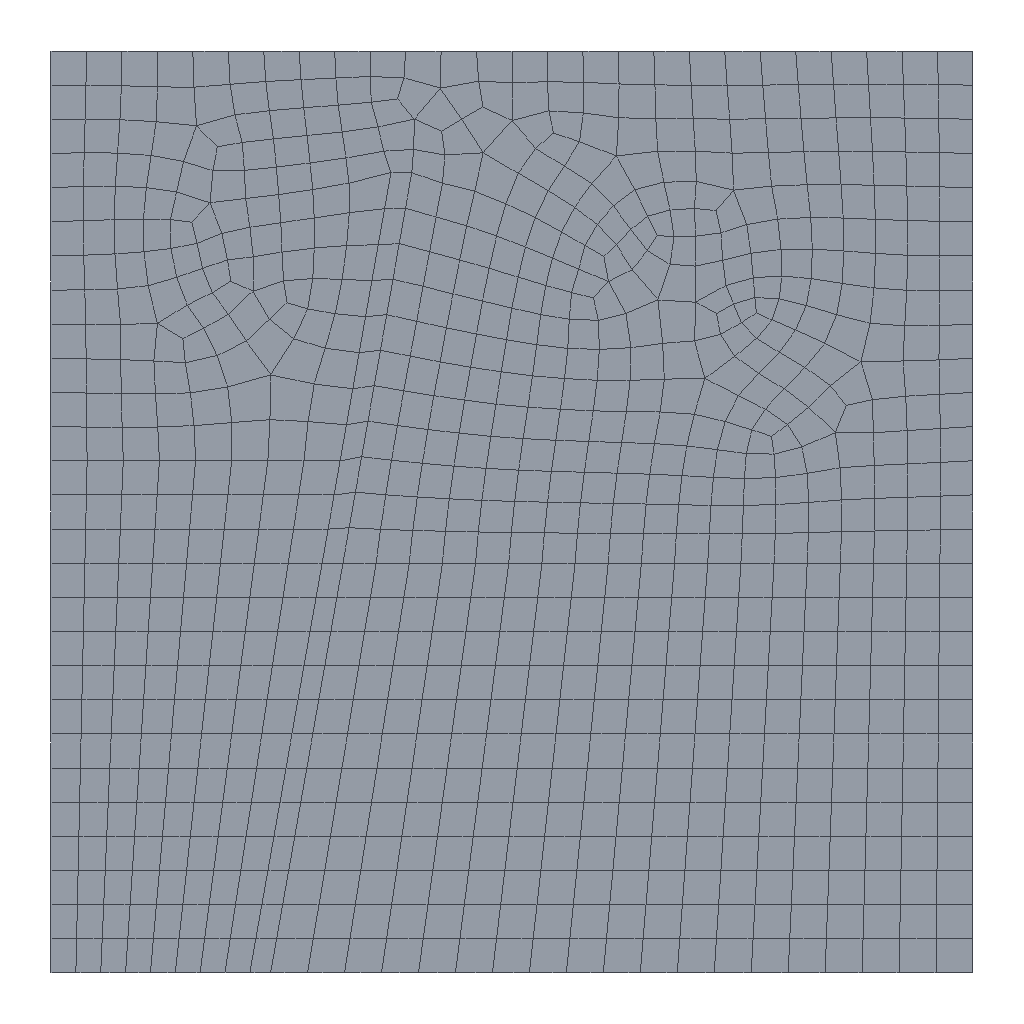Simulation study | abaqus
Set-up summary:
category,name,step,type,value,unit,region
solver,abaqus
solver,version,,,Abaqus/Standard 2020
units,not stated in the deck,,not stated
analysis,deck,,soils,soils
load_step,Step-1,Step-1,soils
load_step,requested,,,1
mesh,nodes,,,855
mesh,elements,,,800
element_type,CPE4P,,plane,800
load,load commands in deck,,count,3
bc,support commands in deck,,count,4
material,CHUSHUI,,in results
material,DUANCENG,,in results
material,SOIL,,in results
check,setup vs results,,match,"per instance, exact: element labels, types and connectivity; labels of the nodes the elements use; coordinates of those nodes at SINGLE_PRECISION in 1 of 1 instance(s)"
Abaqus input file, long lists of numbers shortened:
*Heading
** Job name: Job-2 Model name: Model-1-Copy
** Generated by: Abaqus/CAE 2020
*Preprint, echo=NO, model=NO, history=NO, contact=NO
**
** PARTS
**
*Part, name=Part-1
*Node
      1,   264.619,        -500.
      2,           0.,        -500.
** (853 more lines like these left out)
*Element, type=CPE4P
 1,   1,  17, 205,  52
 2,  17,  18, 206, 205
** (798 more lines like these left out)
*Nset, nset=Set-1
  1,  5, 53, 54
*Elset, elset=Set-1
 104, 112, 120, 133, 134, 135
*Nset, nset=Set-2
   1,   2,   3,   4,   5,   6,   7,   8,   9,  10,  11,  14,  15,  16,  17,  18
  19,  20,  21,  22,  23,  24,  25,  26,  27,  28,  29,  30,  31,  32,  33,  34
** (37 more lines like these left out)
*Elset, elset=Set-2
   1,   2,   3,   4,   5,   6,   7,   8,   9,  10,  11,  12,  13,  14,  15,  16
  17,  18,  19,  20,  21,  22,  23,  24,  25,  26,  27,  28,  29,  30,  31,  32
** (33 more lines like these left out)
*Nset, nset=Set-3
   1,   2,   5,   6,   8,   9,  12,  14,  17,  18,  19,  20,  21,  22,  23,  53
  54,  55,  56,  57,  58,  59,  60,  61,  62,  63,  72,  73,  91,  92,  93,  94
** (6 more lines like these left out)
*Elset, elset=Set-3
  97,  98,  99, 100, 101, 102, 103, 104, 105, 106, 107, 108, 109, 110, 111, 112
 113, 114, 115, 116, 117, 118, 119, 120, 315, 316, 317, 318, 319, 320, 321, 322
** (4 more lines like these left out)
*Nset, nset=Set-4
   7,   8,  12,  13,  64,  65,  66,  67,  68,  69,  70,  71,  91,  92,  93,  94
  95,  96,  97,  98,  99, 100, 101, 102, 103, 104, 105, 106, 107, 108, 109, 110
** (11 more lines like these left out)
*Elset, elset=Set-4, generate
 144,  314,    1
** Section: Section-soil
*Solid Section, elset=Set-2, material=soil
,
** Section: chushui
*Solid Section, elset=Set-3, material=chushui
,
** Section: duanceng
*Solid Section, elset=Set-4, material=duanceng
,
*End Part
**
**
** ASSEMBLY
**
*Assembly, name=Assembly
**
*Instance, name=Part-1-1, part=Part-1
*End Instance
**
*Nset, nset=Set-1, instance=Part-1-1
   1,   5,   6,   8,   9,  10,  16,  53,  54,  72,  73,  74,  75,  76,  77,  78
  79,  80,  81,  82,  83, 194, 195, 196, 197, 198, 199, 200, 201, 202, 203, 204
*Elset, elset=Set-1, instance=Part-1-1
 104, 112, 120, 130, 131, 132, 133, 134, 135, 136, 137, 138, 139, 140, 141, 142
 143, 315, 334, 353, 377, 382, 422, 424, 426, 427, 428, 430, 433, 434, 454, 465
** (1 more lines like these left out)
*Nset, nset=Set-2, instance=Part-1-1
   1,   4,   6,   9,  14,  16,  42,  43,  44,  45,  46,  47,  48,  49,  50,  51
  52, 137, 138, 139, 140, 141, 142, 143, 144, 145, 146, 147, 148, 149, 150, 151
** (1 more lines like these left out)
*Elset, elset=Set-2, instance=Part-1-1
   1,   9,  17,  25,  33,  41,  49,  57,  65,  73,  81,  89, 121, 122, 123, 124
 125, 126, 127, 128, 129, 130, 131, 132, 353, 354, 355, 356, 357, 358, 359, 360
** (3 more lines like these left out)
*Nset, nset=Set-3, instance=Part-1-1
  1,  5,  6, 10, 11, 53, 54, 55, 56, 57, 58, 59, 60, 61
*Elset, elset=Set-3, instance=Part-1-1
 104, 112, 113, 114, 115, 116, 117, 118, 119, 120, 133, 134, 135, 143, 417, 431
 432, 434, 439, 440, 472, 551, 554
*Nset, nset=Set-4, instance=Part-1-1
   1,   5,   6,   9,  10,  16,  53,  54,  74,  75,  76,  77,  78,  79,  80,  81
  82,  83, 194, 195, 196, 197, 198, 199, 200, 201, 202, 203, 204
*Elset, elset=Set-4, instance=Part-1-1
 104, 112, 120, 133, 134, 135, 136, 137, 138, 139, 140, 141, 142, 143, 377, 382
 422, 424, 426, 427, 428, 430, 433, 434, 454, 465, 467, 468, 470, 473, 476, 492
** (1 more lines like these left out)
*Nset, nset=Set-5, instance=Part-1-1
   7,  13,  14,  15, 109, 110, 111, 112, 113, 114, 115, 116, 117, 118, 119, 120
 121, 122, 123, 124, 125, 126, 155, 156, 157, 158, 159, 160, 161, 162, 163, 164
** (1 more lines like these left out)
*Elset, elset=Set-5, instance=Part-1-1
 296, 297, 298, 299, 300, 301, 302, 303, 304, 305, 306, 307, 308, 309, 310, 311
 312, 313, 314, 387, 388, 393, 394, 398, 401, 402, 403, 404, 406, 460, 462, 463
** (1 more lines like these left out)
*Nset, nset=Set-6, instance=Part-1-1
   9,  14, 137, 138, 139, 140, 141, 142, 143, 144, 145, 146, 147, 148, 149, 150
 151, 152, 153, 154
*Elset, elset=Set-6, instance=Part-1-1
 353, 354, 355, 356, 357, 358, 359, 360, 361, 362, 363, 364, 365, 366, 367, 368
 369, 370, 371, 373, 375, 378, 386, 390, 391, 392, 393, 395, 409, 446, 448, 449
** (1 more lines like these left out)
*Nset, nset=Set-7, instance=Part-1-1, generate
   1,  855,    1
*Elset, elset=Set-7, instance=Part-1-1, generate
   1,  800,    1
*Nset, nset=Set-8, instance=Part-1-1
   1,   3,   4,   8,   9,  10,  12,  14,  35,  36,  37,  38,  39,  40,  41,  42
  43,  44,  45,  46,  47,  48,  49,  50,  51,  52,  74,  75,  76,  77,  78,  79
** (3 more lines like these left out)
*Elset, elset=Set-8, instance=Part-1-1
   1,   9,  17,  25,  33,  41,  49,  57,  65,  73,  81,  89,  90,  91,  92,  93
  94,  95,  96, 121, 122, 123, 124, 125, 126, 127, 128, 129, 130, 131, 132, 133
** (6 more lines like these left out)
*Nset, nset=Set-9, instance=Part-1-1
   8,   9,  14,  15,  72,  73, 155, 156, 157, 158, 159, 160, 161, 162, 163, 164
 165, 166, 167, 168
*Elset, elset=Set-9, instance=Part-1-1
 130, 131, 132, 315, 334, 353, 387, 388, 393, 394, 398, 401, 402, 403, 404, 406
 460, 462, 463, 486, 510
*Nset, nset=Set-10, instance=Part-1-1
  1,  5, 10, 11, 53, 54
*Elset, elset=Set-10, instance=Part-1-1
 104, 112, 120, 133, 134, 135, 143, 417
*Nset, nset=Set-11, instance=Part-1-1
  1,  5, 53, 54
*Elset, elset=Set-11, instance=Part-1-1
 104, 112, 120, 133, 134, 135
*Nset, nset=Set-12, instance=Part-1-1, generate
   1,  855,    1
*Elset, elset=Set-12, instance=Part-1-1, generate
   1,  800,    1
*Nset, nset=Set-13, instance=Part-1-1
  1,  5, 53, 54
*Elset, elset=Set-13, instance=Part-1-1
 104, 112, 120, 133, 134, 135
*Nset, nset=Set-14, instance=Part-1-1
  1,  5, 53, 54
*Elset, elset=Set-14, instance=Part-1-1
 104, 112, 120, 133, 134, 135
*Nset, nset=Set-15, instance=Part-1-1
 10, 11
*Elset, elset=Set-15, instance=Part-1-1
 143, 417
*Nset, nset=Set-16, instance=Part-1-1
  1,  5, 10, 11, 53, 54
*Elset, elset=Set-16, instance=Part-1-1
 104, 112, 120, 133, 134, 135, 143, 417
*Nset, nset=Set-17, instance=Part-1-1
 1, 5
*Nset, nset=Set-18, instance=Part-1-1
  1,  5, 53, 54
*Elset, elset=Set-18, instance=Part-1-1
 104, 112, 120, 133, 134, 135
*Nset, nset=Set-19, instance=Part-1-1
 10, 11
*Elset, elset=Set-19, instance=Part-1-1
 143, 417
*Nset, nset=Set-20, instance=Part-1-1
  1,  5, 53, 54
*Elset, elset=Set-20, instance=Part-1-1
 104, 112, 120, 133, 134, 135
*Nset, nset=Set-21, instance=Part-1-1
  1,  2,  5,  6, 53, 54, 62, 63
*Elset, elset=Set-21, instance=Part-1-1
  97, 104, 105, 112, 113, 120, 133, 134, 135
*Nset, nset=Set-22, instance=Part-1-1
  1,  5, 10, 11, 53, 54
*Elset, elset=Set-22, instance=Part-1-1
 104, 112, 120, 133, 134, 135, 143, 417
*Nset, nset=Set-23, instance=Part-1-1
  1,  5, 10, 11, 53, 54
*Elset, elset=Set-23, instance=Part-1-1
 104, 112, 120, 133, 134, 135, 143, 417
*Nset, nset=Set-24, instance=Part-1-1
  1,  5, 53, 54
*Elset, elset=Set-24, instance=Part-1-1
 104, 112, 120, 133, 134, 135
*Nset, nset=Set-25, instance=Part-1-1
  1,  5, 10, 11, 53, 54
*Elset, elset=Set-25, instance=Part-1-1
 104, 112, 120, 133, 134, 135, 143, 417
*Nset, nset=Set-26, instance=Part-1-1
  1,  5, 53, 54
*Elset, elset=Set-26, instance=Part-1-1
 104, 112, 120, 133, 134, 135
*Nset, nset=Set-27, instance=Part-1-1
  1,  5, 10, 11, 53, 54
*Elset, elset=Set-27, instance=Part-1-1
 104, 112, 120, 133, 134, 135, 143, 417
*Nset, nset=Set-28, instance=Part-1-1
  15,  16, 169, 170, 171, 172, 173, 174, 175, 176, 177, 178, 179, 180, 181, 182
 183, 184, 185, 186, 187, 188, 189, 190, 191, 192, 193
*Elset, elset=Set-28, instance=Part-1-1
 399, 404, 405, 412, 413, 414, 415, 420, 425, 426, 444, 487, 490, 491, 493, 507
 512, 513, 520, 525, 527, 531, 532, 533, 601, 603
*Nset, nset=Set-29, instance=Part-1-1
  1,  5, 53, 54
*Elset, elset=Set-29, instance=Part-1-1
 104, 112, 120, 133, 134, 135
*Nset, nset=Set-30, instance=Part-1-1
  1,  5,  8,  9, 53, 54, 72, 73
*Elset, elset=Set-30, instance=Part-1-1
 104, 112, 120, 130, 131, 132, 133, 134, 135, 315, 334, 353
*Nset, nset=Set-31, instance=Part-1-1
   2,   3,   6,  12,  13,  14,  15,  16,  24,  25,  26,  27,  28,  29,  30,  31
  32,  33,  34,  62,  63, 127, 128, 129, 130, 131, 132, 133, 134, 135, 136, 155
** (2 more lines like these left out)
*Elset, elset=Set-31, instance=Part-1-1
   8,  16,  24,  32,  40,  48,  56,  64,  72,  80,  88,  96,  97, 105, 113, 144
 163, 182, 201, 220, 239, 258, 277, 296, 333, 352, 371, 377, 387, 388, 393, 394
** (2 more lines like these left out)
*Nset, nset=Set-32, instance=Part-1-1
   3,   4,   7,  13,  35,  36,  37,  38,  39,  40,  41, 109, 110, 111, 112, 113
 114, 115, 116, 117, 118, 119, 120, 121, 122, 123, 124, 125, 126
*Elset, elset=Set-32, instance=Part-1-1
  89,  90,  91,  92,  93,  94,  95,  96, 121, 296, 297, 298, 299, 300, 301, 302
 303, 304, 305, 306, 307, 308, 309, 310, 311, 312, 313, 314
*Nset, nset=Set-33, instance=Part-1-1
  1,  5, 53, 54
*Elset, elset=Set-33, instance=Part-1-1
 104, 112, 120, 133, 134, 135
*Nset, nset=Set-34, instance=Part-1-1
  1,  5,  8,  9, 53, 54, 72, 73
*Elset, elset=Set-34, instance=Part-1-1
 104, 112, 120, 130, 131, 132, 133, 134, 135, 315, 334, 353
*Nset, nset=Set-35, instance=Part-1-1
 10, 11
*Nset, nset=Set-36, instance=Part-1-1
  1,  5, 53, 54
*Elset, elset=Set-36, instance=Part-1-1
 104, 112, 120, 133, 134, 135
*Nset, nset=Set-37, instance=Part-1-1
  15,  16, 169, 170, 171, 172, 173, 174, 175, 176, 177, 178, 179, 180, 181, 182
 183, 184, 185, 186, 187, 188, 189, 190, 191, 192, 193
*Elset, elset=Set-37, instance=Part-1-1
 143, 399, 404, 405, 412, 413, 414, 415, 417, 420, 425, 426, 444, 487, 490, 491
 493, 507, 512, 513, 520, 525, 527, 531, 532, 533, 601, 603
*Nset, nset=Set-38, instance=Part-1-1
  15,  16, 169, 170, 171, 172, 173, 174, 175, 176, 177, 178, 179, 180, 181, 182
 183, 184, 185, 186, 187, 188, 189, 190, 191, 192, 193
*Elset, elset=Set-38, instance=Part-1-1
 143, 399, 404, 405, 412, 413, 414, 415, 417, 420, 425, 426, 444, 487, 490, 491
 493, 507, 512, 513, 520, 525, 527, 531, 532, 533, 601, 603
*Elset, elset=Set-39, instance=Part-1-1
 143, 417
*Nset, nset=Set-40, instance=Part-1-1
  1,  5,  8,  9, 53, 54, 72, 73
*Elset, elset=Set-40, instance=Part-1-1
 104, 112, 120, 130, 131, 132, 133, 134, 135, 315, 334, 353
*Nset, nset=Set-41, instance=Part-1-1
  15,  16, 169, 170, 171, 172, 173, 174, 175, 176, 177, 178, 179, 180, 181, 182
 183, 184, 185, 186, 187, 188, 189, 190, 191, 192, 193
*Elset, elset=Set-41, instance=Part-1-1
 399, 404, 405, 412, 413, 414, 415, 420, 425, 426, 444, 487, 490, 491, 493, 507
 512, 513, 520, 525, 527, 531, 532, 533, 601, 603
*Nset, nset=Set-42, instance=Part-1-1
  1,  5, 53, 54
*Elset, elset=Set-42, instance=Part-1-1
 104, 112, 120, 133, 134, 135
*Nset, nset=Set-43, instance=Part-1-1
 10, 11
*Elset, elset=Set-43, instance=Part-1-1
 143, 417
*Nset, nset=Set-44, instance=Part-1-1
  1,  5,  8,  9, 53, 54, 72, 73
*Elset, elset=Set-44, instance=Part-1-1
 104, 112, 120, 130, 131, 132, 133, 134, 135, 315, 334, 353
*Nset, nset=Set-45, instance=Part-1-1
  15,  16, 169, 170, 171, 172, 173, 174, 175, 176, 177, 178, 179, 180, 181, 182
 183, 184, 185, 186, 187, 188, 189, 190, 191, 192, 193
*Elset, elset=Set-45, instance=Part-1-1
 143, 399, 404, 405, 412, 413, 414, 415, 417, 420, 425, 426, 444, 487, 490, 491
 493, 507, 512, 513, 520, 525, 527, 531, 532, 533, 601, 603
*Nset, nset=Set-46, instance=Part-1-1
 10, 11
*Elset, elset=Set-46, instance=Part-1-1
 143, 417
*Nset, nset=Set-47, instance=Part-1-1
  15,  16, 169, 170, 171, 172, 173, 174, 175, 176, 177, 178, 179, 180, 181, 182
 183, 184, 185, 186, 187, 188, 189, 190, 191, 192, 193
*Elset, elset=Set-47, instance=Part-1-1
 399, 404, 405, 412, 413, 414, 415, 420, 425, 426, 444, 487, 490, 491, 493, 507
 512, 513, 520, 525, 527, 531, 532, 533, 601, 603
*Elset, elset=_Surf-1_S2, internal, instance=Part-1-1
 373, 378, 386, 390, 446, 448, 454, 456, 459
*Elset, elset=_Surf-1_S4, internal, instance=Part-1-1
 375, 391, 392, 393, 395, 409, 449, 451, 453, 458
*Surface, type=ELEMENT, name=Surf-1
_Surf-1_S2, S2
_Surf-1_S4, S4
*Elset, elset=_Surf-2_S2, internal, instance=Part-1-1, generate
 104,  120,    8
*Elset, elset=_Surf-2_S4, internal, instance=Part-1-1
 417,
*Surface, type=ELEMENT, name=Surf-2
_Surf-2_S2, S2
_Surf-2_S4, S4
*Elset, elset=_Surf-3_S2, internal, instance=Part-1-1, generate
 104,  120,    8
*Surface, type=ELEMENT, name=Surf-3
_Surf-3_S2, S2
*Elset, elset=_Surf-4_S2, internal, instance=Part-1-1, generate
 104,  120,    8
*Elset, elset=_Surf-4_S4, internal, instance=Part-1-1
 417,
*Surface, type=ELEMENT, name=Surf-4
_Surf-4_S2, S2
_Surf-4_S4, S4
*Elset, elset=_Surf-5_S2, internal, instance=Part-1-1, generate
 104,  120,    8
*Surface, type=ELEMENT, name=Surf-5
_Surf-5_S2, S2
*Elset, elset=_Surf-6_S2, internal, instance=Part-1-1, generate
 104,  120,    8
*Elset, elset=_Surf-6_S4, internal, instance=Part-1-1
 417,
*Surface, type=ELEMENT, name=Surf-6
_Surf-6_S2, S2
_Surf-6_S4, S4
*Elset, elset=_Surf-7_S2, internal, instance=Part-1-1, generate
 104,  120,    8
*Surface, type=ELEMENT, name=Surf-7
_Surf-7_S2, S2
*Elset, elset=_Surf-8_S2, internal, instance=Part-1-1, generate
 104,  120,    8
*Elset, elset=_Surf-8_S4, internal, instance=Part-1-1
 417,
*Surface, type=ELEMENT, name=Surf-8
_Surf-8_S2, S2
_Surf-8_S4, S4
*Elset, elset=_Surf-9_S3, internal, instance=Part-1-1
 399, 405, 413, 414, 415, 420, 444, 487, 493, 507, 513, 601, 603
*Elset, elset=_Surf-9_S4, internal, instance=Part-1-1
 404, 425
*Elset, elset=_Surf-9_S1, internal, instance=Part-1-1
 412, 426, 490, 491, 512, 520, 525, 527, 531, 532, 533
*Surface, type=ELEMENT, name=Surf-9
_Surf-9_S3, S3
_Surf-9_S4, S4
_Surf-9_S1, S1
*Nset, nset=Set-44_PP_, internal, instance=Part-1-1
  1,  5,  8,  9, 53, 54, 72, 73
*Nset, nset=Set-47_PP_, internal, instance=Part-1-1
  15,  16, 169, 170, 171, 172, 173, 174, 175, 176, 177, 178, 179, 180, 181, 182
 183, 184, 185, 186, 187, 188, 189, 190, 191, 192, 193
*End Assembly
*Amplitude, name=Amp-1
             0.,              0.,              1.,              1.
**
** MATERIALS
**
*Material, name=chushui
*Density
2200.,
*Elastic
 1.44e+10, 0.2
*Gap Flow
 0.001,
*Permeability, specific=9980.
 1.5e-13, 0.19
*Material, name=duanceng
*Density
2200.,
*Elastic
 1.44e+10, 0.2
*Gap Flow
 0.001,
*Permeability, specific=9980.
 1.5e-09, 0.19
*Material, name=soil
*Density
2500.,
*Elastic
 2.964e+10, 0.12
*Gap Flow
 0.001,
*Permeability, specific=9980.
 2e-16, 0.04
**
** BOUNDARY CONDITIONS
**
** Name: BC-1 Type: 位移/转角
*Boundary
Set-31, 1, 1
** Name: BC-2 Type: 位移/转角
*Boundary
Set-32, 2, 2
**
** PREDEFINED FIELDS
**
** Name: Predefined Field-1   Type: Stress
*Initial Conditions, type=STRESS
Set-7, 0., 0., 0., 0.,
** Name: Predefined Field-2   Type: Void ratio
*Initial Conditions, TYPE=RATIO
Set-12, 1.
** ----------------------------------------------------------------
**
** STEP: Step-1
**
*Step, name=Step-1, nlgeom=YES, inc=1000
*Soils, utol=1.0, creep=none, stabilize=0.0002, allsdtol=0.05, continue=NO
0.01, 1., 1e-05, 1.,
**
** BOUNDARY CONDITIONS
**
** Name: BC-4 Type: 孔隙压力
*Boundary
Set-44_PP_, 8, 8, 1e+08
** Name: [REDACTED] : Pore pressure
*Boundary
Set-47_PP_, 8, 8, 3e+06
**
** LOADS
**
** Name: Load-pressure   Type: Pressure
*Dsload
Surf-9, P, 7.36e+06
**
** OUTPUT REQUESTS
**
*Restart, write, frequency=0
**
** FIELD OUTPUT: F-Output-1
**
*Output, field
*Node Output
CF, POR, RF, U, V
*Element Output, directions=YES
E, FLUVR, FLVEL, LE, MISES, MISESMAX, PE, S, SAT, VOIDR, PEEQ
*Contact Output
PFL, PFLA, PTL, PTLA
**
** HISTORY OUTPUT: H-Output-1
**
*Output, history, variable=PRESELECT
*End Step
Results summary:
result,step,,completed,increments=11 time=1.0/1.0
result,analysis,,,soils
result,last_loadstep,,,1
result,primary field,,,"U, POR"
result,reaction total,,FX,-1724779.5,model units
result,reaction total,,FY,6624027712.0,model units
result,reaction total,,FZ,0.0,model units